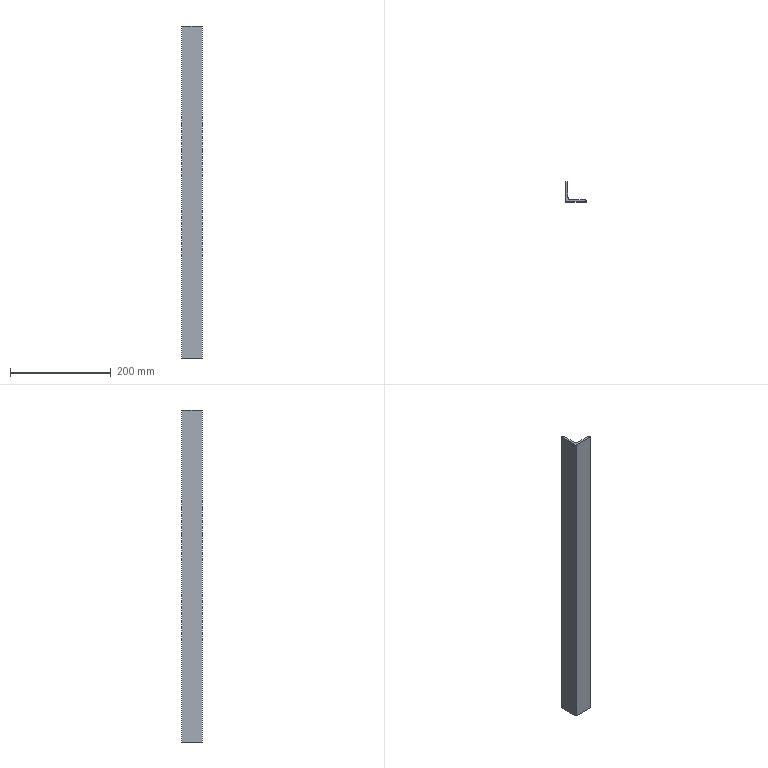Part | SolidWorks | features Extrusion 1 | 1 solid | 11 faces | box 40 x 40 x 660 mm | volume 203677 mm3 | plane 8 | cylinder 3 | commonest cylinder face diameters 2.667 x2 10 x1
STEP:
#1=CARTESIAN_POINT('',(9.,4.,0.));
#2=VERTEX_POINT('',#1);
#3=CARTESIAN_POINT('',(4.,9.,0.));
#4=VERTEX_POINT('',#3);
#5=CARTESIAN_POINT('',(9.,9.,0.));
#6=DIRECTION('',(0.,0.,-1.));
#7=DIRECTION('',(-1.,0.,0.));
#8=AXIS2_PLACEMENT_3D('',#5,#6,#7);
#9=CIRCLE('',#8,5.);
#10=EDGE_CURVE('',#2,#4,#9,.T.);
#11=ORIENTED_EDGE('',*,*,#10,.T.);
#12=CARTESIAN_POINT('',(4.,9.,660.));
#13=VERTEX_POINT('',#12);
#14=CARTESIAN_POINT('',(4.,9.,660.));
#15=DIRECTION('',(0.,0.,-1.));
#16=VECTOR('',#15,1000.);
#17=LINE('',#14,#16);
#18=EDGE_CURVE('',#13,#4,#17,.T.);
#19=ORIENTED_EDGE('',*,*,#18,.F.);
#20=CARTESIAN_POINT('',(9.,4.,660.));
#21=VERTEX_POINT('',#20);
#22=CARTESIAN_POINT('',(9.,9.,660.));
#23=DIRECTION('',(0.,0.,-1.));
#24=DIRECTION('',(-1.,0.,0.));
#25=AXIS2_PLACEMENT_3D('',#22,#23,#24);
#26=CIRCLE('',#25,5.);
#27=EDGE_CURVE('',#21,#13,#26,.T.);
#28=ORIENTED_EDGE('',*,*,#27,.F.);
#29=CARTESIAN_POINT('',(9.,4.,660.));
#30=DIRECTION('',(0.,0.,-1.));
#31=VECTOR('',#30,1000.);
#32=LINE('',#29,#31);
#33=EDGE_CURVE('',#21,#2,#32,.T.);
#34=ORIENTED_EDGE('',*,*,#33,.T.);
#35=EDGE_LOOP('',(#11,#19,#28,#34));
#36=FACE_OUTER_BOUND('',#35,.T.);
#37=CARTESIAN_POINT('',(9.,9.,660.));
#38=DIRECTION('',(0.,0.,-1.));
#39=DIRECTION('',(-1.,0.,0.));
#40=AXIS2_PLACEMENT_3D('',#37,#38,#39);
#41=CYLINDRICAL_SURFACE('',#40,5.);
#42=ADVANCED_FACE('',(#36),#41,.F.);
#43=CARTESIAN_POINT('',(4.,38.667,0.));
#44=VERTEX_POINT('',#43);
#45=CARTESIAN_POINT('',(4.,38.667,0.));
#46=DIRECTION('',(0.,-1.,0.));
#47=VECTOR('',#46,1000.);
#48=LINE('',#45,#47);
#49=EDGE_CURVE('',#44,#4,#48,.T.);
#50=ORIENTED_EDGE('',*,*,#49,.F.);
#51=CARTESIAN_POINT('',(4.,38.667,660.));
#52=VERTEX_POINT('',#51);
#53=CARTESIAN_POINT('',(4.,38.667,660.));
#54=DIRECTION('',(0.,0.,-1.));
#55=VECTOR('',#54,1000.);
#56=LINE('',#53,#55);
#57=EDGE_CURVE('',#52,#44,#56,.T.);
#58=ORIENTED_EDGE('',*,*,#57,.F.);
#59=CARTESIAN_POINT('',(4.,38.667,660.));
#60=DIRECTION('',(0.,-1.,0.));
#61=VECTOR('',#60,1000.);
#62=LINE('',#59,#61);
#63=EDGE_CURVE('',#52,#13,#62,.T.);
#64=ORIENTED_EDGE('',*,*,#63,.T.);
#65=ORIENTED_EDGE('',*,*,#18,.T.);
#66=EDGE_LOOP('',(#50,#58,#64,#65));
#67=FACE_OUTER_BOUND('',#66,.T.);
#68=CARTESIAN_POINT('',(4.,38.667,660.));
#69=DIRECTION('',(1.,0.,0.));
#70=DIRECTION('',(0.,1.,0.));
#71=AXIS2_PLACEMENT_3D('',#68,#69,#70);
#72=PLANE('',#71);
#73=ADVANCED_FACE('',(#67),#72,.T.);
#74=CARTESIAN_POINT('',(2.667,40.,0.));
#75=VERTEX_POINT('',#74);
#76=CARTESIAN_POINT('',(2.667,38.667,0.));
#77=DIRECTION('',(0.,0.,-1.));
#78=DIRECTION('',(-1.,0.,0.));
#79=AXIS2_PLACEMENT_3D('',#76,#77,#78);
#80=CIRCLE('',#79,1.333);
#81=EDGE_CURVE('',#75,#44,#80,.T.);
#82=ORIENTED_EDGE('',*,*,#81,.F.);
#83=CARTESIAN_POINT('',(2.667,40.,660.));
#84=VERTEX_POINT('',#83);
#85=CARTESIAN_POINT('',(2.667,40.,660.));
#86=DIRECTION('',(0.,0.,-1.));
#87=VECTOR('',#86,1000.);
#88=LINE('',#85,#87);
#89=EDGE_CURVE('',#84,#75,#88,.T.);
#90=ORIENTED_EDGE('',*,*,#89,.F.);
#91=CARTESIAN_POINT('',(2.667,38.667,660.));
#92=DIRECTION('',(0.,0.,-1.));
#93=DIRECTION('',(-1.,0.,0.));
#94=AXIS2_PLACEMENT_3D('',#91,#92,#93);
#95=CIRCLE('',#94,1.333);
#96=EDGE_CURVE('',#84,#52,#95,.T.);
#97=ORIENTED_EDGE('',*,*,#96,.T.);
#98=ORIENTED_EDGE('',*,*,#57,.T.);
#99=EDGE_LOOP('',(#82,#90,#97,#98));
#100=FACE_OUTER_BOUND('',#99,.T.);
#101=CARTESIAN_POINT('',(2.667,38.667,660.));
#102=DIRECTION('',(0.,0.,-1.));
#103=DIRECTION('',(-1.,0.,0.));
#104=AXIS2_PLACEMENT_3D('',#101,#102,#103);
#105=CYLINDRICAL_SURFACE('',#104,1.333);
#106=ADVANCED_FACE('',(#100),#105,.T.);
#107=CARTESIAN_POINT('',(0.,40.,0.));
#108=VERTEX_POINT('',#107);
#109=CARTESIAN_POINT('',(0.,40.,0.));
#110=DIRECTION('',(1.,0.,0.));
#111=VECTOR('',#110,1000.);
#112=LINE('',#109,#111);
#113=EDGE_CURVE('',#108,#75,#112,.T.);
#114=ORIENTED_EDGE('',*,*,#113,.F.);
#115=CARTESIAN_POINT('',(0.,40.,660.));
#116=VERTEX_POINT('',#115);
#117=CARTESIAN_POINT('',(0.,40.,660.));
#118=DIRECTION('',(0.,0.,-1.));
#119=VECTOR('',#118,1000.);
#120=LINE('',#117,#119);
#121=EDGE_CURVE('',#116,#108,#120,.T.);
#122=ORIENTED_EDGE('',*,*,#121,.F.);
#123=CARTESIAN_POINT('',(0.,40.,660.));
#124=DIRECTION('',(1.,0.,0.));
#125=VECTOR('',#124,1000.);
#126=LINE('',#123,#125);
#127=EDGE_CURVE('',#116,#84,#126,.T.);
#128=ORIENTED_EDGE('',*,*,#127,.T.);
#129=ORIENTED_EDGE('',*,*,#89,.T.);
#130=EDGE_LOOP('',(#114,#122,#128,#129));
#131=FACE_OUTER_BOUND('',#130,.T.);
#132=CARTESIAN_POINT('',(0.,40.,660.));
#133=DIRECTION('',(0.,1.,0.));
#134=DIRECTION('',(0.,0.,1.));
#135=AXIS2_PLACEMENT_3D('',#132,#133,#134);
#136=PLANE('',#135);
#137=ADVANCED_FACE('',(#131),#136,.T.);
#138=CARTESIAN_POINT('',(0.,0.,0.));
#139=VERTEX_POINT('',#138);
#140=CARTESIAN_POINT('',(0.,0.,0.));
#141=DIRECTION('',(0.,1.,0.));
#142=VECTOR('',#141,1000.);
#143=LINE('',#140,#142);
#144=EDGE_CURVE('',#139,#108,#143,.T.);
#145=ORIENTED_EDGE('',*,*,#144,.F.);
#146=CARTESIAN_POINT('',(0.,0.,660.));
#147=VERTEX_POINT('',#146);
#148=CARTESIAN_POINT('',(0.,0.,660.));
#149=DIRECTION('',(0.,0.,-1.));
#150=VECTOR('',#149,1000.);
#151=LINE('',#148,#150);
#152=EDGE_CURVE('',#147,#139,#151,.T.);
#153=ORIENTED_EDGE('',*,*,#152,.F.);
#154=CARTESIAN_POINT('',(0.,0.,660.));
#155=DIRECTION('',(0.,1.,0.));
#156=VECTOR('',#155,1000.);
#157=LINE('',#154,#156);
#158=EDGE_CURVE('',#147,#116,#157,.T.);
#159=ORIENTED_EDGE('',*,*,#158,.T.);
#160=ORIENTED_EDGE('',*,*,#121,.T.);
#161=EDGE_LOOP('',(#145,#153,#159,#160));
#162=FACE_OUTER_BOUND('',#161,.T.);
#163=CARTESIAN_POINT('',(0.,0.,660.));
#164=DIRECTION('',(-1.,0.,0.));
#165=DIRECTION('',(0.,0.,1.));
#166=AXIS2_PLACEMENT_3D('',#163,#164,#165);
#167=PLANE('',#166);
#168=ADVANCED_FACE('',(#162),#167,.T.);
#169=CARTESIAN_POINT('',(40.,0.,0.));
#170=VERTEX_POINT('',#169);
#171=CARTESIAN_POINT('',(40.,0.,0.));
#172=DIRECTION('',(-1.,0.,0.));
#173=VECTOR('',#172,1000.);
#174=LINE('',#171,#173);
#175=EDGE_CURVE('',#170,#139,#174,.T.);
#176=ORIENTED_EDGE('',*,*,#175,.F.);
#177=CARTESIAN_POINT('',(40.,0.,660.));
#178=VERTEX_POINT('',#177);
#179=CARTESIAN_POINT('',(40.,0.,660.));
#180=DIRECTION('',(0.,0.,-1.));
#181=VECTOR('',#180,1000.);
#182=LINE('',#179,#181);
#183=EDGE_CURVE('',#178,#170,#182,.T.);
#184=ORIENTED_EDGE('',*,*,#183,.F.);
#185=CARTESIAN_POINT('',(40.,0.,660.));
#186=DIRECTION('',(-1.,0.,0.));
#187=VECTOR('',#186,1000.);
#188=LINE('',#185,#187);
#189=EDGE_CURVE('',#178,#147,#188,.T.);
#190=ORIENTED_EDGE('',*,*,#189,.T.);
#191=ORIENTED_EDGE('',*,*,#152,.T.);
#192=EDGE_LOOP('',(#176,#184,#190,#191));
#193=FACE_OUTER_BOUND('',#192,.T.);
#194=CARTESIAN_POINT('',(40.,0.,660.));
#195=DIRECTION('',(0.,-1.,0.));
#196=DIRECTION('',(0.,0.,-1.));
#197=AXIS2_PLACEMENT_3D('',#194,#195,#196);
#198=PLANE('',#197);
#199=ADVANCED_FACE('',(#193),#198,.T.);
#200=CARTESIAN_POINT('',(40.,2.667,0.));
#201=VERTEX_POINT('',#200);
#202=CARTESIAN_POINT('',(40.,0.,0.));
#203=DIRECTION('',(0.,1.,0.));
#204=VECTOR('',#203,1000.);
#205=LINE('',#202,#204);
#206=EDGE_CURVE('',#170,#201,#205,.T.);
#207=ORIENTED_EDGE('',*,*,#206,.T.);
#208=CARTESIAN_POINT('',(40.,2.667,660.));
#209=VERTEX_POINT('',#208);
#210=CARTESIAN_POINT('',(40.,2.667,660.));
#211=DIRECTION('',(0.,0.,-1.));
#212=VECTOR('',#211,1000.);
#213=LINE('',#210,#212);
#214=EDGE_CURVE('',#209,#201,#213,.T.);
#215=ORIENTED_EDGE('',*,*,#214,.F.);
#216=CARTESIAN_POINT('',(40.,0.,660.));
#217=DIRECTION('',(0.,1.,0.));
#218=VECTOR('',#217,1000.);
#219=LINE('',#216,#218);
#220=EDGE_CURVE('',#178,#209,#219,.T.);
#221=ORIENTED_EDGE('',*,*,#220,.F.);
#222=ORIENTED_EDGE('',*,*,#183,.T.);
#223=EDGE_LOOP('',(#207,#215,#221,#222));
#224=FACE_OUTER_BOUND('',#223,.T.);
#225=CARTESIAN_POINT('',(40.,0.,660.));
#226=DIRECTION('',(-1.,0.,0.));
#227=DIRECTION('',(0.,-1.,0.));
#228=AXIS2_PLACEMENT_3D('',#225,#226,#227);
#229=PLANE('',#228);
#230=ADVANCED_FACE('',(#224),#229,.F.);
#231=CARTESIAN_POINT('',(38.667,4.,0.));
#232=VERTEX_POINT('',#231);
#233=CARTESIAN_POINT('',(38.667,2.667,0.));
#234=DIRECTION('',(0.,0.,1.));
#235=DIRECTION('',(1.,0.,0.));
#236=AXIS2_PLACEMENT_3D('',#233,#234,#235);
#237=CIRCLE('',#236,1.333);
#238=EDGE_CURVE('',#201,#232,#237,.T.);
#239=ORIENTED_EDGE('',*,*,#238,.T.);
#240=CARTESIAN_POINT('',(38.667,4.,660.));
#241=VERTEX_POINT('',#240);
#242=CARTESIAN_POINT('',(38.667,4.,660.));
#243=DIRECTION('',(0.,0.,-1.));
#244=VECTOR('',#243,1000.);
#245=LINE('',#242,#244);
#246=EDGE_CURVE('',#241,#232,#245,.T.);
#247=ORIENTED_EDGE('',*,*,#246,.F.);
#248=CARTESIAN_POINT('',(38.667,2.667,660.));
#249=DIRECTION('',(0.,0.,1.));
#250=DIRECTION('',(1.,0.,0.));
#251=AXIS2_PLACEMENT_3D('',#248,#249,#250);
#252=CIRCLE('',#251,1.333);
#253=EDGE_CURVE('',#209,#241,#252,.T.);
#254=ORIENTED_EDGE('',*,*,#253,.F.);
#255=ORIENTED_EDGE('',*,*,#214,.T.);
#256=EDGE_LOOP('',(#239,#247,#254,#255));
#257=FACE_OUTER_BOUND('',#256,.T.);
#258=CARTESIAN_POINT('',(38.667,2.667,660.));
#259=DIRECTION('',(0.,0.,-1.));
#260=DIRECTION('',(-1.,0.,0.));
#261=AXIS2_PLACEMENT_3D('',#258,#259,#260);
#262=CYLINDRICAL_SURFACE('',#261,1.333);
#263=ADVANCED_FACE('',(#257),#262,.T.);
#264=CARTESIAN_POINT('',(9.,4.,0.));
#265=DIRECTION('',(1.,0.,0.));
#266=VECTOR('',#265,1000.);
#267=LINE('',#264,#266);
#268=EDGE_CURVE('',#2,#232,#267,.T.);
#269=ORIENTED_EDGE('',*,*,#268,.F.);
#270=ORIENTED_EDGE('',*,*,#33,.F.);
#271=CARTESIAN_POINT('',(9.,4.,660.));
#272=DIRECTION('',(1.,0.,0.));
#273=VECTOR('',#272,1000.);
#274=LINE('',#271,#273);
#275=EDGE_CURVE('',#21,#241,#274,.T.);
#276=ORIENTED_EDGE('',*,*,#275,.T.);
#277=ORIENTED_EDGE('',*,*,#246,.T.);
#278=EDGE_LOOP('',(#269,#270,#276,#277));
#279=FACE_OUTER_BOUND('',#278,.T.);
#280=CARTESIAN_POINT('',(9.,4.,660.));
#281=DIRECTION('',(0.,1.,0.));
#282=DIRECTION('',(-1.,0.,0.));
#283=AXIS2_PLACEMENT_3D('',#280,#281,#282);
#284=PLANE('',#283);
#285=ADVANCED_FACE('',(#279),#284,.T.);
#286=ORIENTED_EDGE('',*,*,#27,.T.);
#287=ORIENTED_EDGE('',*,*,#63,.F.);
#288=ORIENTED_EDGE('',*,*,#96,.F.);
#289=ORIENTED_EDGE('',*,*,#127,.F.);
#290=ORIENTED_EDGE('',*,*,#158,.F.);
#291=ORIENTED_EDGE('',*,*,#189,.F.);
#292=ORIENTED_EDGE('',*,*,#220,.T.);
#293=ORIENTED_EDGE('',*,*,#253,.T.);
#294=ORIENTED_EDGE('',*,*,#275,.F.);
#295=EDGE_LOOP('',(#286,#287,#288,#289,#290,#291,#292,#293,#294));
#296=FACE_OUTER_BOUND('',#295,.T.);
#297=CARTESIAN_POINT('',(9.,9.,660.));
#298=DIRECTION('',(0.,0.,-1.));
#299=DIRECTION('',(-1.,0.,0.));
#300=AXIS2_PLACEMENT_3D('',#297,#298,#299);
#301=PLANE('',#300);
#302=ADVANCED_FACE('',(#296),#301,.F.);
#303=ORIENTED_EDGE('',*,*,#10,.F.);
#304=ORIENTED_EDGE('',*,*,#268,.T.);
#305=ORIENTED_EDGE('',*,*,#238,.F.);
#306=ORIENTED_EDGE('',*,*,#206,.F.);
#307=ORIENTED_EDGE('',*,*,#175,.T.);
#308=ORIENTED_EDGE('',*,*,#144,.T.);
#309=ORIENTED_EDGE('',*,*,#113,.T.);
#310=ORIENTED_EDGE('',*,*,#81,.T.);
#311=ORIENTED_EDGE('',*,*,#49,.T.);
#312=EDGE_LOOP('',(#303,#304,#305,#306,#307,#308,#309,#310,#311));
#313=FACE_OUTER_BOUND('',#312,.T.);
#314=CARTESIAN_POINT('',(9.,9.,0.));
#315=DIRECTION('',(0.,0.,-1.));
#316=DIRECTION('',(-1.,0.,0.));
#317=AXIS2_PLACEMENT_3D('',#314,#315,#316);
#318=PLANE('',#317);
#319=ADVANCED_FACE('',(#313),#318,.T.);
#320=CLOSED_SHELL('',(#42,#73,#106,#137,#168,#199,#230,#263,#285,#302,#319));
#321=MANIFOLD_SOLID_BREP('',#320);
#322=CARTESIAN_POINT('',(0.,0.,0.));
#323=DIRECTION('',(0.,0.,1.));
#324=DIRECTION('',(1.,0.,0.));
#325=AXIS2_PLACEMENT_3D('',#322,#323,#324);
#326=(LENGTH_UNIT()NAMED_UNIT(*)SI_UNIT(.MILLI.,.METRE.));
#327=UNCERTAINTY_MEASURE_WITH_UNIT(LENGTH_MEASURE(0.00001),#326,'','');
#328=(NAMED_UNIT(*)PLANE_ANGLE_UNIT()SI_UNIT($,.RADIAN.));
#329=(NAMED_UNIT(*)SI_UNIT($,.STERADIAN.)SOLID_ANGLE_UNIT());
#330=(GEOMETRIC_REPRESENTATION_CONTEXT(3)GLOBAL_UNCERTAINTY_ASSIGNED_CONTEXT((#327))GLOBAL_UNIT_ASSIGNED_CONTEXT((#326,#328,#329))REPRESENTATION_CONTEXT('',''));
#331=ADVANCED_BREP_SHAPE_REPRESENTATION('',(#321,#325),#330);